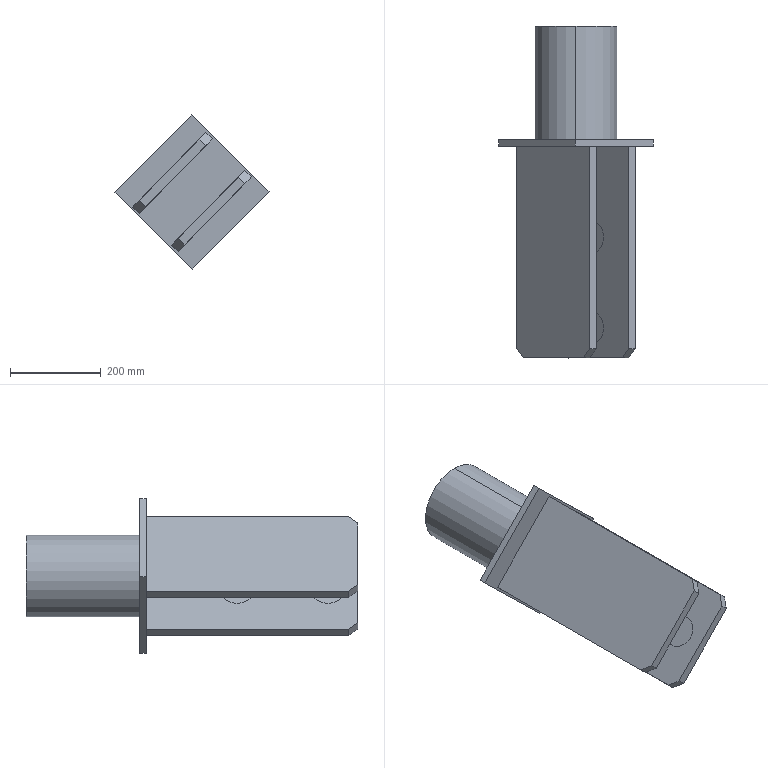Part | SolidWorks | features BaseBody 1 | 1 solid | 35 faces | box 339.392 x 731.247 x 339.392 mm | volume 11422226 mm3 | plane 25 | cylinder 10 | commonest cylinder face diameters 70 x8 180 x2
STEP:
#1=CARTESIAN_POINT('',(14.827,1234.2,-1080.412));
#2=VERTEX_POINT('',#1);
#3=CARTESIAN_POINT('',(63.788,1234.2,-1030.384));
#4=VERTEX_POINT('',#3);
#5=CARTESIAN_POINT('',(39.308,1234.2,-1055.398));
#6=DIRECTION('',(-0.7147,0.,0.6994));
#7=DIRECTION('',(0.6994,0.,0.7147));
#8=AXIS2_PLACEMENT_3D('',#5,#6,#7);
#9=CIRCLE('',#8,35.);
#10=EDGE_CURVE('',#2,#4,#9,.T.);
#11=ORIENTED_EDGE('',*,*,#10,.F.);
#12=CARTESIAN_POINT('',(11.254,1234.2,-1076.915));
#13=VERTEX_POINT('',#12);
#14=CARTESIAN_POINT('',(14.827,1234.2,-1080.412));
#15=DIRECTION('',(-0.7147,0.,0.6994));
#16=VECTOR('',#15,1000.);
#17=LINE('',#14,#16);
#18=EDGE_CURVE('',#2,#13,#17,.T.);
#19=ORIENTED_EDGE('',*,*,#18,.T.);
#20=CARTESIAN_POINT('',(60.215,1234.2,-1026.887));
#21=VERTEX_POINT('',#20);
#22=CARTESIAN_POINT('',(35.734,1234.2,-1051.901));
#23=DIRECTION('',(-0.7147,0.,0.6994));
#24=DIRECTION('',(0.6994,0.,0.7147));
#25=AXIS2_PLACEMENT_3D('',#22,#23,#24);
#26=CIRCLE('',#25,35.);
#27=EDGE_CURVE('',#13,#21,#26,.T.);
#28=ORIENTED_EDGE('',*,*,#27,.T.);
#29=CARTESIAN_POINT('',(63.788,1234.2,-1030.384));
#30=DIRECTION('',(-0.7147,0.,0.6994));
#31=VECTOR('',#30,1000.);
#32=LINE('',#29,#31);
#33=EDGE_CURVE('',#4,#21,#32,.T.);
#34=ORIENTED_EDGE('',*,*,#33,.F.);
#35=EDGE_LOOP('',(#11,#19,#28,#34));
#36=FACE_OUTER_BOUND('',#35,.T.);
#37=CARTESIAN_POINT('',(39.308,1234.2,-1055.398));
#38=DIRECTION('',(-0.7147,0.,0.6994));
#39=DIRECTION('',(0.6994,0.,0.7147));
#40=AXIS2_PLACEMENT_3D('',#37,#38,#39);
#41=CYLINDRICAL_SURFACE('',#40,35.);
#42=ADVANCED_FACE('',(#36),#41,.F.);
#43=CARTESIAN_POINT('',(14.827,1034.2,-1080.412));
#44=VERTEX_POINT('',#43);
#45=CARTESIAN_POINT('',(63.788,1034.2,-1030.384));
#46=VERTEX_POINT('',#45);
#47=CARTESIAN_POINT('',(39.308,1034.2,-1055.398));
#48=DIRECTION('',(-0.7147,0.,0.6994));
#49=DIRECTION('',(0.6994,0.,0.7147));
#50=AXIS2_PLACEMENT_3D('',#47,#48,#49);
#51=CIRCLE('',#50,35.);
#52=EDGE_CURVE('',#44,#46,#51,.T.);
#53=ORIENTED_EDGE('',*,*,#52,.F.);
#54=CARTESIAN_POINT('',(11.254,1034.2,-1076.915));
#55=VERTEX_POINT('',#54);
#56=CARTESIAN_POINT('',(14.827,1034.2,-1080.412));
#57=DIRECTION('',(-0.7147,0.,0.6994));
#58=VECTOR('',#57,1000.);
#59=LINE('',#56,#58);
#60=EDGE_CURVE('',#44,#55,#59,.T.);
#61=ORIENTED_EDGE('',*,*,#60,.T.);
#62=CARTESIAN_POINT('',(60.215,1034.2,-1026.887));
#63=VERTEX_POINT('',#62);
#64=CARTESIAN_POINT('',(35.734,1034.2,-1051.901));
#65=DIRECTION('',(-0.7147,0.,0.6994));
#66=DIRECTION('',(0.6994,0.,0.7147));
#67=AXIS2_PLACEMENT_3D('',#64,#65,#66);
#68=CIRCLE('',#67,35.);
#69=EDGE_CURVE('',#55,#63,#68,.T.);
#70=ORIENTED_EDGE('',*,*,#69,.T.);
#71=CARTESIAN_POINT('',(63.788,1034.2,-1030.384));
#72=DIRECTION('',(-0.7147,0.,0.6994));
#73=VECTOR('',#72,1000.);
#74=LINE('',#71,#73);
#75=EDGE_CURVE('',#46,#63,#74,.T.);
#76=ORIENTED_EDGE('',*,*,#75,.F.);
#77=EDGE_LOOP('',(#53,#61,#70,#76));
#78=FACE_OUTER_BOUND('',#77,.T.);
#79=CARTESIAN_POINT('',(39.308,1034.2,-1055.398));
#80=DIRECTION('',(-0.7147,0.,0.6994));
#81=DIRECTION('',(0.6994,0.,0.7147));
#82=AXIS2_PLACEMENT_3D('',#79,#80,#81);
#83=CYLINDRICAL_SURFACE('',#82,35.);
#84=ADVANCED_FACE('',(#78),#83,.F.);
#85=CARTESIAN_POINT('',(-14.827,1034.2,-953.445));
#86=VERTEX_POINT('',#85);
#87=CARTESIAN_POINT('',(-63.788,1034.2,-1003.473));
#88=VERTEX_POINT('',#87);
#89=CARTESIAN_POINT('',(-39.308,1034.2,-978.459));
#90=DIRECTION('',(0.7147,0.,-0.6994));
#91=DIRECTION('',(-0.6994,0.,-0.7147));
#92=AXIS2_PLACEMENT_3D('',#89,#90,#91);
#93=CIRCLE('',#92,35.);
#94=EDGE_CURVE('',#86,#88,#93,.T.);
#95=ORIENTED_EDGE('',*,*,#94,.F.);
#96=CARTESIAN_POINT('',(-11.254,1034.2,-956.942));
#97=VERTEX_POINT('',#96);
#98=CARTESIAN_POINT('',(-14.827,1034.2,-953.445));
#99=DIRECTION('',(0.7147,0.,-0.6994));
#100=VECTOR('',#99,1000.);
#101=LINE('',#98,#100);
#102=EDGE_CURVE('',#86,#97,#101,.T.);
#103=ORIENTED_EDGE('',*,*,#102,.T.);
#104=CARTESIAN_POINT('',(-60.215,1034.2,-1006.971));
#105=VERTEX_POINT('',#104);
#106=CARTESIAN_POINT('',(-35.734,1034.2,-981.957));
#107=DIRECTION('',(0.7147,0.,-0.6994));
#108=DIRECTION('',(-0.6994,0.,-0.7147));
#109=AXIS2_PLACEMENT_3D('',#106,#107,#108);
#110=CIRCLE('',#109,35.);
#111=EDGE_CURVE('',#97,#105,#110,.T.);
#112=ORIENTED_EDGE('',*,*,#111,.T.);
#113=CARTESIAN_POINT('',(-63.788,1034.2,-1003.473));
#114=DIRECTION('',(0.7147,0.,-0.6994));
#115=VECTOR('',#114,1000.);
#116=LINE('',#113,#115);
#117=EDGE_CURVE('',#88,#105,#116,.T.);
#118=ORIENTED_EDGE('',*,*,#117,.F.);
#119=EDGE_LOOP('',(#95,#103,#112,#118));
#120=FACE_OUTER_BOUND('',#119,.T.);
#121=CARTESIAN_POINT('',(-39.308,1034.2,-978.459));
#122=DIRECTION('',(0.7147,0.,-0.6994));
#123=DIRECTION('',(-0.6994,0.,-0.7147));
#124=AXIS2_PLACEMENT_3D('',#121,#122,#123);
#125=CYLINDRICAL_SURFACE('',#124,35.);
#126=ADVANCED_FACE('',(#120),#125,.F.);
#127=CARTESIAN_POINT('',(-14.827,1234.2,-953.445));
#128=VERTEX_POINT('',#127);
#129=CARTESIAN_POINT('',(-63.788,1234.2,-1003.473));
#130=VERTEX_POINT('',#129);
#131=CARTESIAN_POINT('',(-39.308,1234.2,-978.459));
#132=DIRECTION('',(0.7147,0.,-0.6994));
#133=DIRECTION('',(-0.6994,0.,-0.7147));
#134=AXIS2_PLACEMENT_3D('',#131,#132,#133);
#135=CIRCLE('',#134,35.);
#136=EDGE_CURVE('',#128,#130,#135,.T.);
#137=ORIENTED_EDGE('',*,*,#136,.F.);
#138=CARTESIAN_POINT('',(-11.254,1234.2,-956.942));
#139=VERTEX_POINT('',#138);
#140=CARTESIAN_POINT('',(-14.827,1234.2,-953.445));
#141=DIRECTION('',(0.7147,0.,-0.6994));
#142=VECTOR('',#141,1000.);
#143=LINE('',#140,#142);
#144=EDGE_CURVE('',#128,#139,#143,.T.);
#145=ORIENTED_EDGE('',*,*,#144,.T.);
#146=CARTESIAN_POINT('',(-60.215,1234.2,-1006.971));
#147=VERTEX_POINT('',#146);
#148=CARTESIAN_POINT('',(-35.734,1234.2,-981.957));
#149=DIRECTION('',(0.7147,0.,-0.6994));
#150=DIRECTION('',(-0.6994,0.,-0.7147));
#151=AXIS2_PLACEMENT_3D('',#148,#149,#150);
#152=CIRCLE('',#151,35.);
#153=EDGE_CURVE('',#139,#147,#152,.T.);
#154=ORIENTED_EDGE('',*,*,#153,.T.);
#155=CARTESIAN_POINT('',(-63.788,1234.2,-1003.473));
#156=DIRECTION('',(0.7147,0.,-0.6994));
#157=VECTOR('',#156,1000.);
#158=LINE('',#155,#157);
#159=EDGE_CURVE('',#130,#147,#158,.T.);
#160=ORIENTED_EDGE('',*,*,#159,.F.);
#161=EDGE_LOOP('',(#137,#145,#154,#160));
#162=FACE_OUTER_BOUND('',#161,.T.);
#163=CARTESIAN_POINT('',(-39.308,1234.2,-978.459));
#164=DIRECTION('',(0.7147,0.,-0.6994));
#165=DIRECTION('',(-0.6994,0.,-0.7147));
#166=AXIS2_PLACEMENT_3D('',#163,#164,#165);
#167=CYLINDRICAL_SURFACE('',#166,35.);
#168=ADVANCED_FACE('',(#162),#167,.F.);
#169=CARTESIAN_POINT('',(0.,1699.2,-1106.929));
#170=VERTEX_POINT('',#169);
#171=CARTESIAN_POINT('',(0.,1699.2,-926.929));
#172=VERTEX_POINT('',#171);
#173=CARTESIAN_POINT('',(0.,1699.2,-1016.929));
#174=DIRECTION('',(0.,-1.,0.));
#175=DIRECTION('',(0.,0.,-1.));
#176=AXIS2_PLACEMENT_3D('',#173,#174,#175);
#177=CIRCLE('',#176,90.);
#178=EDGE_CURVE('',#170,#172,#177,.T.);
#179=ORIENTED_EDGE('',*,*,#178,.T.);
#180=CARTESIAN_POINT('',(0.,1449.2,-926.929));
#181=VERTEX_POINT('',#180);
#182=CARTESIAN_POINT('',(0.,1699.2,-926.929));
#183=DIRECTION('',(0.,-1.,0.));
#184=VECTOR('',#183,1000.);
#185=LINE('',#182,#184);
#186=EDGE_CURVE('',#172,#181,#185,.T.);
#187=ORIENTED_EDGE('',*,*,#186,.T.);
#188=CARTESIAN_POINT('',(0.,1449.2,-1106.929));
#189=VERTEX_POINT('',#188);
#190=CARTESIAN_POINT('',(0.,1449.2,-1016.929));
#191=DIRECTION('',(0.,1.,0.));
#192=DIRECTION('',(0.,0.,-1.));
#193=AXIS2_PLACEMENT_3D('',#190,#191,#192);
#194=CIRCLE('',#193,90.);
#195=EDGE_CURVE('',#181,#189,#194,.T.);
#196=ORIENTED_EDGE('',*,*,#195,.T.);
#197=CARTESIAN_POINT('',(0.,1699.2,-1106.929));
#198=DIRECTION('',(0.,-1.,0.));
#199=VECTOR('',#198,1000.);
#200=LINE('',#197,#199);
#201=EDGE_CURVE('',#170,#189,#200,.T.);
#202=ORIENTED_EDGE('',*,*,#201,.F.);
#203=EDGE_LOOP('',(#179,#187,#196,#202));
#204=FACE_OUTER_BOUND('',#203,.T.);
#205=CARTESIAN_POINT('',(0.,1699.2,-1016.929));
#206=DIRECTION('',(0.,-1.,0.));
#207=DIRECTION('',(0.,0.,-1.));
#208=AXIS2_PLACEMENT_3D('',#205,#206,#207);
#209=CYLINDRICAL_SURFACE('',#208,90.);
#210=ADVANCED_FACE('',(#204),#209,.T.);
#211=CARTESIAN_POINT('',(-30.408,987.953,-1148.079));
#212=VERTEX_POINT('',#211);
#213=CARTESIAN_POINT('',(-16.419,967.953,-1133.785));
#214=VERTEX_POINT('',#213);
#215=CARTESIAN_POINT('',(-30.408,987.953,-1148.079));
#216=DIRECTION('',(0.4946,-0.7071,0.5054));
#217=VECTOR('',#216,1000.);
#218=LINE('',#215,#217);
#219=EDGE_CURVE('',#212,#214,#218,.T.);
#220=ORIENTED_EDGE('',*,*,#219,.F.);
#221=CARTESIAN_POINT('',(-30.408,1434.2,-1148.079));
#222=VERTEX_POINT('',#221);
#223=CARTESIAN_POINT('',(-30.408,864.2,-1148.079));
#224=DIRECTION('',(0.,-1.,0.));
#225=VECTOR('',#224,1000.);
#226=LINE('',#223,#225);
#227=EDGE_CURVE('',#222,#212,#226,.T.);
#228=ORIENTED_EDGE('',*,*,#227,.F.);
#229=CARTESIAN_POINT('',(130.464,1434.2,-983.701));
#230=VERTEX_POINT('',#229);
#231=CARTESIAN_POINT('',(-30.408,1434.2,-1148.079));
#232=DIRECTION('',(-0.6994,0.,-0.7147));
#233=VECTOR('',#232,1000.);
#234=LINE('',#231,#233);
#235=EDGE_CURVE('',#230,#222,#234,.T.);
#236=ORIENTED_EDGE('',*,*,#235,.F.);
#237=CARTESIAN_POINT('',(130.464,987.953,-983.701));
#238=VERTEX_POINT('',#237);
#239=CARTESIAN_POINT('',(130.464,864.2,-983.701));
#240=DIRECTION('',(0.,1.,0.));
#241=VECTOR('',#240,1000.);
#242=LINE('',#239,#241);
#243=EDGE_CURVE('',#238,#230,#242,.T.);
#244=ORIENTED_EDGE('',*,*,#243,.F.);
#245=CARTESIAN_POINT('',(116.475,967.953,-997.995));
#246=VERTEX_POINT('',#245);
#247=CARTESIAN_POINT('',(116.475,967.953,-997.995));
#248=DIRECTION('',(0.4946,0.7071,0.5054));
#249=VECTOR('',#248,1000.);
#250=LINE('',#247,#249);
#251=EDGE_CURVE('',#246,#238,#250,.T.);
#252=ORIENTED_EDGE('',*,*,#251,.F.);
#253=CARTESIAN_POINT('',(-30.408,967.953,-1148.079));
#254=DIRECTION('',(0.6994,0.,0.7147));
#255=VECTOR('',#254,1000.);
#256=LINE('',#253,#255);
#257=EDGE_CURVE('',#214,#246,#256,.T.);
#258=ORIENTED_EDGE('',*,*,#257,.F.);
#259=EDGE_LOOP('',(#220,#228,#236,#244,#252,#258));
#260=FACE_OUTER_BOUND('',#259,.T.);
#261=CARTESIAN_POINT('',(-30.408,864.2,-1148.079));
#262=DIRECTION('',(-0.7147,0.,0.6994));
#263=DIRECTION('',(0.6994,0.,0.7147));
#264=AXIS2_PLACEMENT_3D('',#261,#262,#263);
#265=PLANE('',#264);
#266=ADVANCED_FACE('',(#260),#265,.F.);
#267=CARTESIAN_POINT('',(-30.713,967.953,-1119.796));
#268=VERTEX_POINT('',#267);
#269=CARTESIAN_POINT('',(-16.419,967.953,-1133.785));
#270=DIRECTION('',(-0.7147,0.,0.6994));
#271=VECTOR('',#270,1000.);
#272=LINE('',#269,#271);
#273=EDGE_CURVE('',#214,#268,#272,.T.);
#274=ORIENTED_EDGE('',*,*,#273,.F.);
#275=ORIENTED_EDGE('',*,*,#257,.T.);
#276=CARTESIAN_POINT('',(102.182,967.953,-984.006));
#277=VERTEX_POINT('',#276);
#278=CARTESIAN_POINT('',(102.182,967.953,-984.006));
#279=DIRECTION('',(0.7147,0.,-0.6994));
#280=VECTOR('',#279,1000.);
#281=LINE('',#278,#280);
#282=EDGE_CURVE('',#277,#246,#281,.T.);
#283=ORIENTED_EDGE('',*,*,#282,.F.);
#284=CARTESIAN_POINT('',(-30.713,967.953,-1119.796));
#285=DIRECTION('',(0.6994,0.,0.7147));
#286=VECTOR('',#285,1000.);
#287=LINE('',#284,#286);
#288=EDGE_CURVE('',#268,#277,#287,.T.);
#289=ORIENTED_EDGE('',*,*,#288,.F.);
#290=EDGE_LOOP('',(#274,#275,#283,#289));
#291=FACE_OUTER_BOUND('',#290,.T.);
#292=CARTESIAN_POINT('',(155.411,967.953,-1329.934));
#293=DIRECTION('',(0.,1.,0.));
#294=DIRECTION('',(0.,0.,1.));
#295=AXIS2_PLACEMENT_3D('',#292,#293,#294);
#296=PLANE('',#295);
#297=ADVANCED_FACE('',(#291),#296,.F.);
#298=ORIENTED_EDGE('',*,*,#273,.T.);
#299=CARTESIAN_POINT('',(-44.702,987.953,-1134.09));
#300=VERTEX_POINT('',#299);
#301=CARTESIAN_POINT('',(-44.702,987.953,-1134.09));
#302=DIRECTION('',(0.4946,-0.7071,0.5054));
#303=VECTOR('',#302,1000.);
#304=LINE('',#301,#303);
#305=EDGE_CURVE('',#300,#268,#304,.T.);
#306=ORIENTED_EDGE('',*,*,#305,.F.);
#307=CARTESIAN_POINT('',(-30.408,987.953,-1148.079));
#308=DIRECTION('',(-0.7147,0.,0.6994));
#309=VECTOR('',#308,1000.);
#310=LINE('',#307,#309);
#311=EDGE_CURVE('',#212,#300,#310,.T.);
#312=ORIENTED_EDGE('',*,*,#311,.F.);
#313=ORIENTED_EDGE('',*,*,#219,.T.);
#314=EDGE_LOOP('',(#298,#306,#312,#313));
#315=FACE_OUTER_BOUND('',#314,.T.);
#316=CARTESIAN_POINT('',(-30.408,987.953,-1148.079));
#317=DIRECTION('',(0.4946,0.7071,0.5054));
#318=DIRECTION('',(0.,-0.5815,0.8136));
#319=AXIS2_PLACEMENT_3D('',#316,#317,#318);
#320=PLANE('',#319);
#321=ADVANCED_FACE('',(#315),#320,.F.);
#322=ORIENTED_EDGE('',*,*,#311,.T.);
#323=CARTESIAN_POINT('',(-44.702,1434.2,-1134.09));
#324=VERTEX_POINT('',#323);
#325=CARTESIAN_POINT('',(-44.702,864.2,-1134.09));
#326=DIRECTION('',(0.,-1.,0.));
#327=VECTOR('',#326,1000.);
#328=LINE('',#325,#327);
#329=EDGE_CURVE('',#324,#300,#328,.T.);
#330=ORIENTED_EDGE('',*,*,#329,.F.);
#331=CARTESIAN_POINT('',(-30.408,1434.2,-1148.079));
#332=DIRECTION('',(-0.7147,0.,0.6994));
#333=VECTOR('',#332,1000.);
#334=LINE('',#331,#333);
#335=EDGE_CURVE('',#222,#324,#334,.T.);
#336=ORIENTED_EDGE('',*,*,#335,.F.);
#337=ORIENTED_EDGE('',*,*,#227,.T.);
#338=EDGE_LOOP('',(#322,#330,#336,#337));
#339=FACE_OUTER_BOUND('',#338,.T.);
#340=CARTESIAN_POINT('',(-30.408,864.2,-1148.079));
#341=DIRECTION('',(0.6994,0.,0.7147));
#342=DIRECTION('',(0.7147,0.,-0.6994));
#343=AXIS2_PLACEMENT_3D('',#340,#341,#342);
#344=PLANE('',#343);
#345=ADVANCED_FACE('',(#339),#344,.F.);
#346=CARTESIAN_POINT('',(-130.464,1434.2,-1050.157));
#347=VERTEX_POINT('',#346);
#348=CARTESIAN_POINT('',(30.408,1434.2,-885.779));
#349=VERTEX_POINT('',#348);
#350=CARTESIAN_POINT('',(-130.464,1434.2,-1050.157));
#351=DIRECTION('',(0.6994,0.,0.7147));
#352=VECTOR('',#351,1000.);
#353=LINE('',#350,#352);
#354=EDGE_CURVE('',#347,#349,#353,.T.);
#355=ORIENTED_EDGE('',*,*,#354,.T.);
#356=CARTESIAN_POINT('',(44.702,1434.2,-899.767));
#357=VERTEX_POINT('',#356);
#358=CARTESIAN_POINT('',(30.408,1434.2,-885.779));
#359=DIRECTION('',(0.7147,0.,-0.6994));
#360=VECTOR('',#359,1000.);
#361=LINE('',#358,#360);
#362=EDGE_CURVE('',#349,#357,#361,.T.);
#363=ORIENTED_EDGE('',*,*,#362,.T.);
#364=CARTESIAN_POINT('',(-116.17,1434.2,-1064.146));
#365=VERTEX_POINT('',#364);
#366=CARTESIAN_POINT('',(44.702,1434.2,-899.767));
#367=DIRECTION('',(-0.6994,0.,-0.7147));
#368=VECTOR('',#367,1000.);
#369=LINE('',#366,#368);
#370=EDGE_CURVE('',#357,#365,#369,.T.);
#371=ORIENTED_EDGE('',*,*,#370,.T.);
#372=CARTESIAN_POINT('',(-116.17,1434.2,-1064.146));
#373=DIRECTION('',(-0.7147,0.,0.6994));
#374=VECTOR('',#373,1000.);
#375=LINE('',#372,#374);
#376=EDGE_CURVE('',#365,#347,#375,.T.);
#377=ORIENTED_EDGE('',*,*,#376,.T.);
#378=EDGE_LOOP('',(#355,#363,#371,#377));
#379=FACE_BOUND('',#378,.T.);
#380=CARTESIAN_POINT('',(-1.829,1434.2,-847.233));
#381=VERTEX_POINT('',#380);
#382=CARTESIAN_POINT('',(-169.696,1434.2,-1018.758));
#383=VERTEX_POINT('',#382);
#384=CARTESIAN_POINT('',(-1.829,1434.2,-847.233));
#385=DIRECTION('',(-0.6994,0.,-0.7147));
#386=VECTOR('',#385,1000.);
#387=LINE('',#384,#386);
#388=EDGE_CURVE('',#381,#383,#387,.T.);
#389=ORIENTED_EDGE('',*,*,#388,.T.);
#390=CARTESIAN_POINT('',(1.829,1434.2,-1186.625));
#391=VERTEX_POINT('',#390);
#392=CARTESIAN_POINT('',(-169.696,1434.2,-1018.758));
#393=DIRECTION('',(0.7147,0.,-0.6994));
#394=VECTOR('',#393,1000.);
#395=LINE('',#392,#394);
#396=EDGE_CURVE('',#383,#391,#395,.T.);
#397=ORIENTED_EDGE('',*,*,#396,.T.);
#398=CARTESIAN_POINT('',(169.696,1434.2,-1015.1));
#399=VERTEX_POINT('',#398);
#400=CARTESIAN_POINT('',(1.829,1434.2,-1186.625));
#401=DIRECTION('',(0.6994,0.,0.7147));
#402=VECTOR('',#401,1000.);
#403=LINE('',#400,#402);
#404=EDGE_CURVE('',#391,#399,#403,.T.);
#405=ORIENTED_EDGE('',*,*,#404,.T.);
#406=CARTESIAN_POINT('',(169.696,1434.2,-1015.1));
#407=DIRECTION('',(-0.7147,0.,0.6994));
#408=VECTOR('',#407,1000.);
#409=LINE('',#406,#408);
#410=EDGE_CURVE('',#399,#381,#409,.T.);
#411=ORIENTED_EDGE('',*,*,#410,.T.);
#412=EDGE_LOOP('',(#389,#397,#405,#411));
#413=FACE_OUTER_BOUND('',#412,.T.);
#414=ORIENTED_EDGE('',*,*,#335,.T.);
#415=CARTESIAN_POINT('',(116.17,1434.2,-969.712));
#416=VERTEX_POINT('',#415);
#417=CARTESIAN_POINT('',(-44.702,1434.2,-1134.09));
#418=DIRECTION('',(0.6994,0.,0.7147));
#419=VECTOR('',#418,1000.);
#420=LINE('',#417,#419);
#421=EDGE_CURVE('',#324,#416,#420,.T.);
#422=ORIENTED_EDGE('',*,*,#421,.T.);
#423=CARTESIAN_POINT('',(116.17,1434.2,-969.712));
#424=DIRECTION('',(0.7147,0.,-0.6994));
#425=VECTOR('',#424,1000.);
#426=LINE('',#423,#425);
#427=EDGE_CURVE('',#416,#230,#426,.T.);
#428=ORIENTED_EDGE('',*,*,#427,.T.);
#429=ORIENTED_EDGE('',*,*,#235,.T.);
#430=EDGE_LOOP('',(#414,#422,#428,#429));
#431=FACE_BOUND('',#430,.T.);
#432=CARTESIAN_POINT('',(0.,1434.2,-1016.929));
#433=DIRECTION('',(0.,-1.,0.));
#434=DIRECTION('',(0.,0.,-1.));
#435=AXIS2_PLACEMENT_3D('',#432,#433,#434);
#436=PLANE('',#435);
#437=ADVANCED_FACE('',(#379,#413,#431),#436,.T.);
#438=CARTESIAN_POINT('',(116.17,987.953,-969.712));
#439=VERTEX_POINT('',#438);
#440=CARTESIAN_POINT('',(130.464,987.953,-983.701));
#441=DIRECTION('',(-0.7147,0.,0.6994));
#442=VECTOR('',#441,1000.);
#443=LINE('',#440,#442);
#444=EDGE_CURVE('',#238,#439,#443,.T.);
#445=ORIENTED_EDGE('',*,*,#444,.F.);
#446=ORIENTED_EDGE('',*,*,#243,.T.);
#447=ORIENTED_EDGE('',*,*,#427,.F.);
#448=CARTESIAN_POINT('',(116.17,864.2,-969.712));
#449=DIRECTION('',(0.,1.,0.));
#450=VECTOR('',#449,1000.);
#451=LINE('',#448,#450);
#452=EDGE_CURVE('',#439,#416,#451,.T.);
#453=ORIENTED_EDGE('',*,*,#452,.F.);
#454=EDGE_LOOP('',(#445,#446,#447,#453));
#455=FACE_OUTER_BOUND('',#454,.T.);
#456=CARTESIAN_POINT('',(130.464,864.2,-983.701));
#457=DIRECTION('',(-0.6994,0.,-0.7147));
#458=DIRECTION('',(-0.7147,0.,0.6994));
#459=AXIS2_PLACEMENT_3D('',#456,#457,#458);
#460=PLANE('',#459);
#461=ADVANCED_FACE('',(#455),#460,.F.);
#462=ORIENTED_EDGE('',*,*,#444,.T.);
#463=CARTESIAN_POINT('',(102.182,967.953,-984.006));
#464=DIRECTION('',(0.4946,0.7071,0.5054));
#465=VECTOR('',#464,1000.);
#466=LINE('',#463,#465);
#467=EDGE_CURVE('',#277,#439,#466,.T.);
#468=ORIENTED_EDGE('',*,*,#467,.F.);
#469=ORIENTED_EDGE('',*,*,#282,.T.);
#470=ORIENTED_EDGE('',*,*,#251,.T.);
#471=EDGE_LOOP('',(#462,#468,#469,#470));
#472=FACE_OUTER_BOUND('',#471,.T.);
#473=CARTESIAN_POINT('',(302.294,967.953,-1179.85));
#474=DIRECTION('',(-0.4946,0.7071,-0.5054));
#475=DIRECTION('',(0.,0.5815,0.8136));
#476=AXIS2_PLACEMENT_3D('',#473,#474,#475);
#477=PLANE('',#476);
#478=ADVANCED_FACE('',(#472),#477,.F.);
#479=CARTESIAN_POINT('',(35.734,1234.2,-1051.901));
#480=DIRECTION('',(-0.7147,0.,0.6994));
#481=DIRECTION('',(0.6994,0.,0.7147));
#482=AXIS2_PLACEMENT_3D('',#479,#480,#481);
#483=CIRCLE('',#482,35.);
#484=EDGE_CURVE('',#21,#13,#483,.T.);
#485=ORIENTED_EDGE('',*,*,#484,.F.);
#486=ORIENTED_EDGE('',*,*,#27,.F.);
#487=EDGE_LOOP('',(#485,#486));
#488=FACE_BOUND('',#487,.T.);
#489=ORIENTED_EDGE('',*,*,#305,.T.);
#490=ORIENTED_EDGE('',*,*,#288,.T.);
#491=ORIENTED_EDGE('',*,*,#467,.T.);
#492=ORIENTED_EDGE('',*,*,#452,.T.);
#493=ORIENTED_EDGE('',*,*,#421,.F.);
#494=ORIENTED_EDGE('',*,*,#329,.T.);
#495=EDGE_LOOP('',(#489,#490,#491,#492,#493,#494));
#496=FACE_OUTER_BOUND('',#495,.T.);
#497=CARTESIAN_POINT('',(35.734,1034.2,-1051.901));
#498=DIRECTION('',(-0.7147,0.,0.6994));
#499=DIRECTION('',(0.6994,0.,0.7147));
#500=AXIS2_PLACEMENT_3D('',#497,#498,#499);
#501=CIRCLE('',#500,35.);
#502=EDGE_CURVE('',#63,#55,#501,.T.);
#503=ORIENTED_EDGE('',*,*,#502,.F.);
#504=ORIENTED_EDGE('',*,*,#69,.F.);
#505=EDGE_LOOP('',(#503,#504));
#506=FACE_BOUND('',#505,.T.);
#507=CARTESIAN_POINT('',(-44.702,864.2,-1134.09));
#508=DIRECTION('',(0.7147,0.,-0.6994));
#509=DIRECTION('',(-0.6994,0.,-0.7147));
#510=AXIS2_PLACEMENT_3D('',#507,#508,#509);
#511=PLANE('',#510);
#512=ADVANCED_FACE('',(#488,#496,#506),#511,.F.);
#513=CARTESIAN_POINT('',(44.702,987.953,-899.767));
#514=VERTEX_POINT('',#513);
#515=CARTESIAN_POINT('',(30.408,987.953,-885.779));
#516=VERTEX_POINT('',#515);
#517=CARTESIAN_POINT('',(30.408,987.953,-885.779));
#518=DIRECTION('',(-0.7147,0.,0.6994));
#519=VECTOR('',#518,1000.);
#520=LINE('',#517,#519);
#521=EDGE_CURVE('',#514,#516,#520,.T.);
#522=ORIENTED_EDGE('',*,*,#521,.F.);
#523=CARTESIAN_POINT('',(44.702,864.2,-899.767));
#524=DIRECTION('',(0.,-1.,0.));
#525=VECTOR('',#524,1000.);
#526=LINE('',#523,#525);
#527=EDGE_CURVE('',#357,#514,#526,.T.);
#528=ORIENTED_EDGE('',*,*,#527,.F.);
#529=ORIENTED_EDGE('',*,*,#362,.F.);
#530=CARTESIAN_POINT('',(30.408,864.2,-885.779));
#531=DIRECTION('',(0.,1.,0.));
#532=VECTOR('',#531,1000.);
#533=LINE('',#530,#532);
#534=EDGE_CURVE('',#516,#349,#533,.T.);
#535=ORIENTED_EDGE('',*,*,#534,.F.);
#536=EDGE_LOOP('',(#522,#528,#529,#535));
#537=FACE_OUTER_BOUND('',#536,.T.);
#538=CARTESIAN_POINT('',(30.408,864.2,-885.779));
#539=DIRECTION('',(-0.6994,0.,-0.7147));
#540=DIRECTION('',(-0.7147,0.,0.6994));
#541=AXIS2_PLACEMENT_3D('',#538,#539,#540);
#542=PLANE('',#541);
#543=ADVANCED_FACE('',(#537),#542,.F.);
#544=CARTESIAN_POINT('',(16.419,967.953,-900.072));
#545=VERTEX_POINT('',#544);
#546=CARTESIAN_POINT('',(30.408,987.953,-885.779));
#547=DIRECTION('',(-0.4946,-0.7071,-0.5054));
#548=VECTOR('',#547,1000.);
#549=LINE('',#546,#548);
#550=EDGE_CURVE('',#516,#545,#549,.T.);
#551=ORIENTED_EDGE('',*,*,#550,.F.);
#552=ORIENTED_EDGE('',*,*,#534,.T.);
#553=ORIENTED_EDGE('',*,*,#354,.F.);
#554=CARTESIAN_POINT('',(-130.464,987.953,-1050.157));
#555=VERTEX_POINT('',#554);
#556=CARTESIAN_POINT('',(-130.464,864.2,-1050.157));
#557=DIRECTION('',(0.,1.,0.));
#558=VECTOR('',#557,1000.);
#559=LINE('',#556,#558);
#560=EDGE_CURVE('',#555,#347,#559,.T.);
#561=ORIENTED_EDGE('',*,*,#560,.F.);
#562=CARTESIAN_POINT('',(-116.475,967.953,-1035.863));
#563=VERTEX_POINT('',#562);
#564=CARTESIAN_POINT('',(-116.475,967.953,-1035.863));
#565=DIRECTION('',(-0.4946,0.7071,-0.5054));
#566=VECTOR('',#565,1000.);
#567=LINE('',#564,#566);
#568=EDGE_CURVE('',#563,#555,#567,.T.);
#569=ORIENTED_EDGE('',*,*,#568,.F.);
#570=CARTESIAN_POINT('',(-130.464,967.953,-1050.157));
#571=DIRECTION('',(-0.6994,0.,-0.7147));
#572=VECTOR('',#571,1000.);
#573=LINE('',#570,#572);
#574=EDGE_CURVE('',#545,#563,#573,.T.);
#575=ORIENTED_EDGE('',*,*,#574,.F.);
#576=EDGE_LOOP('',(#551,#552,#553,#561,#569,#575));
#577=FACE_OUTER_BOUND('',#576,.T.);
#578=CARTESIAN_POINT('',(-130.464,864.2,-1050.157));
#579=DIRECTION('',(0.7147,0.,-0.6994));
#580=DIRECTION('',(-0.6994,0.,-0.7147));
#581=AXIS2_PLACEMENT_3D('',#578,#579,#580);
#582=PLANE('',#581);
#583=ADVANCED_FACE('',(#577),#582,.F.);
#584=CARTESIAN_POINT('',(-116.17,987.953,-1064.146));
#585=VERTEX_POINT('',#584);
#586=CARTESIAN_POINT('',(-130.464,987.953,-1050.157));
#587=DIRECTION('',(0.7147,0.,-0.6994));
#588=VECTOR('',#587,1000.);
#589=LINE('',#586,#588);
#590=EDGE_CURVE('',#555,#585,#589,.T.);
#591=ORIENTED_EDGE('',*,*,#590,.F.);
#592=ORIENTED_EDGE('',*,*,#560,.T.);
#593=ORIENTED_EDGE('',*,*,#376,.F.);
#594=CARTESIAN_POINT('',(-116.17,864.2,-1064.146));
#595=DIRECTION('',(0.,1.,0.));
#596=VECTOR('',#595,1000.);
#597=LINE('',#594,#596);
#598=EDGE_CURVE('',#585,#365,#597,.T.);
#599=ORIENTED_EDGE('',*,*,#598,.F.);
#600=EDGE_LOOP('',(#591,#592,#593,#599));
#601=FACE_OUTER_BOUND('',#600,.T.);
#602=CARTESIAN_POINT('',(-130.464,864.2,-1050.157));
#603=DIRECTION('',(0.6994,0.,0.7147));
#604=DIRECTION('',(0.7147,0.,-0.6994));
#605=AXIS2_PLACEMENT_3D('',#602,#603,#604);
#606=PLANE('',#605);
#607=ADVANCED_FACE('',(#601),#606,.F.);
#608=CARTESIAN_POINT('',(30.713,967.953,-914.061));
#609=VERTEX_POINT('',#608);
#610=CARTESIAN_POINT('',(30.713,967.953,-914.061));
#611=DIRECTION('',(0.4946,0.7071,0.5054));
#612=VECTOR('',#611,1000.);
#613=LINE('',#610,#612);
#614=EDGE_CURVE('',#609,#514,#613,.T.);
#615=ORIENTED_EDGE('',*,*,#614,.F.);
#616=CARTESIAN_POINT('',(-102.182,967.953,-1049.852));
#617=VERTEX_POINT('',#616);
#618=CARTESIAN_POINT('',(-116.17,967.953,-1064.146));
#619=DIRECTION('',(0.6994,0.,0.7147));
#620=VECTOR('',#619,1000.);
#621=LINE('',#618,#620);
#622=EDGE_CURVE('',#617,#609,#621,.T.);
#623=ORIENTED_EDGE('',*,*,#622,.F.);
#624=CARTESIAN_POINT('',(-116.17,987.953,-1064.146));
#625=DIRECTION('',(0.4946,-0.7071,0.5054));
#626=VECTOR('',#625,1000.);
#627=LINE('',#624,#626);
#628=EDGE_CURVE('',#585,#617,#627,.T.);
#629=ORIENTED_EDGE('',*,*,#628,.F.);
#630=ORIENTED_EDGE('',*,*,#598,.T.);
#631=ORIENTED_EDGE('',*,*,#370,.F.);
#632=ORIENTED_EDGE('',*,*,#527,.T.);
#633=EDGE_LOOP('',(#615,#623,#629,#630,#631,#632));
#634=FACE_OUTER_BOUND('',#633,.T.);
#635=CARTESIAN_POINT('',(-35.734,1034.2,-981.957));
#636=DIRECTION('',(0.7147,0.,-0.6994));
#637=DIRECTION('',(-0.6994,0.,-0.7147));
#638=AXIS2_PLACEMENT_3D('',#635,#636,#637);
#639=CIRCLE('',#638,35.);
#640=EDGE_CURVE('',#105,#97,#639,.T.);
#641=ORIENTED_EDGE('',*,*,#640,.F.);
#642=ORIENTED_EDGE('',*,*,#111,.F.);
#643=EDGE_LOOP('',(#641,#642));
#644=FACE_BOUND('',#643,.T.);
#645=CARTESIAN_POINT('',(-35.734,1234.2,-981.957));
#646=DIRECTION('',(0.7147,0.,-0.6994));
#647=DIRECTION('',(-0.6994,0.,-0.7147));
#648=AXIS2_PLACEMENT_3D('',#645,#646,#647);
#649=CIRCLE('',#648,35.);
#650=EDGE_CURVE('',#147,#139,#649,.T.);
#651=ORIENTED_EDGE('',*,*,#650,.F.);
#652=ORIENTED_EDGE('',*,*,#153,.F.);
#653=EDGE_LOOP('',(#651,#652));
#654=FACE_BOUND('',#653,.T.);
#655=CARTESIAN_POINT('',(-116.17,864.2,-1064.146));
#656=DIRECTION('',(-0.7147,0.,0.6994));
#657=DIRECTION('',(0.6994,0.,0.7147));
#658=AXIS2_PLACEMENT_3D('',#655,#656,#657);
#659=PLANE('',#658);
#660=ADVANCED_FACE('',(#634,#644,#654),#659,.F.);
#661=CARTESIAN_POINT('',(1.829,1449.2,-1186.625));
#662=VERTEX_POINT('',#661);
#663=CARTESIAN_POINT('',(1.829,1434.2,-1186.625));
#664=DIRECTION('',(0.,1.,0.));
#665=VECTOR('',#664,1000.);
#666=LINE('',#663,#665);
#667=EDGE_CURVE('',#391,#662,#666,.T.);
#668=ORIENTED_EDGE('',*,*,#667,.F.);
#669=ORIENTED_EDGE('',*,*,#396,.F.);
#670=CARTESIAN_POINT('',(-169.696,1449.2,-1018.758));
#671=VERTEX_POINT('',#670);
#672=CARTESIAN_POINT('',(-169.696,1434.2,-1018.758));
#673=DIRECTION('',(0.,-1.,0.));
#674=VECTOR('',#673,1000.);
#675=LINE('',#672,#674);
#676=EDGE_CURVE('',#671,#383,#675,.T.);
#677=ORIENTED_EDGE('',*,*,#676,.F.);
#678=CARTESIAN_POINT('',(1.829,1449.2,-1186.625));
#679=DIRECTION('',(-0.7147,0.,0.6994));
#680=VECTOR('',#679,1000.);
#681=LINE('',#678,#680);
#682=EDGE_CURVE('',#662,#671,#681,.T.);
#683=ORIENTED_EDGE('',*,*,#682,.F.);
#684=EDGE_LOOP('',(#668,#669,#677,#683));
#685=FACE_OUTER_BOUND('',#684,.T.);
#686=CARTESIAN_POINT('',(1.829,1434.2,-1186.625));
#687=DIRECTION('',(0.6994,0.,0.7147));
#688=DIRECTION('',(0.7147,0.,-0.6994));
#689=AXIS2_PLACEMENT_3D('',#686,#687,#688);
#690=PLANE('',#689);
#691=ADVANCED_FACE('',(#685),#690,.F.);
#692=ORIENTED_EDGE('',*,*,#676,.T.);
#693=ORIENTED_EDGE('',*,*,#388,.F.);
#694=CARTESIAN_POINT('',(-1.829,1449.2,-847.233));
#695=VERTEX_POINT('',#694);
#696=CARTESIAN_POINT('',(-1.829,1434.2,-847.233));
#697=DIRECTION('',(0.,-1.,0.));
#698=VECTOR('',#697,1000.);
#699=LINE('',#696,#698);
#700=EDGE_CURVE('',#695,#381,#699,.T.);
#701=ORIENTED_EDGE('',*,*,#700,.F.);
#702=CARTESIAN_POINT('',(-169.696,1449.2,-1018.758));
#703=DIRECTION('',(0.6994,0.,0.7147));
#704=VECTOR('',#703,1000.);
#705=LINE('',#702,#704);
#706=EDGE_CURVE('',#671,#695,#705,.T.);
#707=ORIENTED_EDGE('',*,*,#706,.F.);
#708=EDGE_LOOP('',(#692,#693,#701,#707));
#709=FACE_OUTER_BOUND('',#708,.T.);
#710=CARTESIAN_POINT('',(-169.696,1434.2,-1018.758));
#711=DIRECTION('',(0.7147,0.,-0.6994));
#712=DIRECTION('',(-0.6994,0.,-0.7147));
#713=AXIS2_PLACEMENT_3D('',#710,#711,#712);
#714=PLANE('',#713);
#715=ADVANCED_FACE('',(#709),#714,.F.);
#716=ORIENTED_EDGE('',*,*,#700,.T.);
#717=ORIENTED_EDGE('',*,*,#410,.F.);
#718=CARTESIAN_POINT('',(169.696,1449.2,-1015.1));
#719=VERTEX_POINT('',#718);
#720=CARTESIAN_POINT('',(169.696,1434.2,-1015.1));
#721=DIRECTION('',(0.,-1.,0.));
#722=VECTOR('',#721,1000.);
#723=LINE('',#720,#722);
#724=EDGE_CURVE('',#719,#399,#723,.T.);
#725=ORIENTED_EDGE('',*,*,#724,.F.);
#726=CARTESIAN_POINT('',(169.696,1449.2,-1015.1));
#727=DIRECTION('',(0.7147,0.,-0.6994));
#728=VECTOR('',#727,1000.);
#729=LINE('',#726,#728);
#730=EDGE_CURVE('',#695,#719,#729,.T.);
#731=ORIENTED_EDGE('',*,*,#730,.F.);
#732=EDGE_LOOP('',(#716,#717,#725,#731));
#733=FACE_OUTER_BOUND('',#732,.T.);
#734=CARTESIAN_POINT('',(169.696,1434.2,-1015.1));
#735=DIRECTION('',(-0.6994,0.,-0.7147));
#736=DIRECTION('',(-0.7147,0.,0.6994));
#737=AXIS2_PLACEMENT_3D('',#734,#735,#736);
#738=PLANE('',#737);
#739=ADVANCED_FACE('',(#733),#738,.F.);
#740=ORIENTED_EDGE('',*,*,#724,.T.);
#741=ORIENTED_EDGE('',*,*,#404,.F.);
#742=ORIENTED_EDGE('',*,*,#667,.T.);
#743=CARTESIAN_POINT('',(1.829,1449.2,-1186.625));
#744=DIRECTION('',(-0.6994,0.,-0.7147));
#745=VECTOR('',#744,1000.);
#746=LINE('',#743,#745);
#747=EDGE_CURVE('',#719,#662,#746,.T.);
#748=ORIENTED_EDGE('',*,*,#747,.F.);
#749=EDGE_LOOP('',(#740,#741,#742,#748));
#750=FACE_OUTER_BOUND('',#749,.T.);
#751=CARTESIAN_POINT('',(1.829,1434.2,-1186.625));
#752=DIRECTION('',(-0.7147,0.,0.6994));
#753=DIRECTION('',(0.6994,0.,0.7147));
#754=AXIS2_PLACEMENT_3D('',#751,#752,#753);
#755=PLANE('',#754);
#756=ADVANCED_FACE('',(#750),#755,.F.);
#757=ORIENTED_EDGE('',*,*,#18,.F.);
#758=CARTESIAN_POINT('',(39.308,1234.2,-1055.398));
#759=DIRECTION('',(-0.7147,0.,0.6994));
#760=DIRECTION('',(0.6994,0.,0.7147));
#761=AXIS2_PLACEMENT_3D('',#758,#759,#760);
#762=CIRCLE('',#761,35.);
#763=EDGE_CURVE('',#4,#2,#762,.T.);
#764=ORIENTED_EDGE('',*,*,#763,.F.);
#765=ORIENTED_EDGE('',*,*,#33,.T.);
#766=ORIENTED_EDGE('',*,*,#484,.T.);
#767=EDGE_LOOP('',(#757,#764,#765,#766));
#768=FACE_OUTER_BOUND('',#767,.T.);
#769=CARTESIAN_POINT('',(39.308,1234.2,-1055.398));
#770=DIRECTION('',(-0.7147,0.,0.6994));
#771=DIRECTION('',(0.6994,0.,0.7147));
#772=AXIS2_PLACEMENT_3D('',#769,#770,#771);
#773=CYLINDRICAL_SURFACE('',#772,35.);
#774=ADVANCED_FACE('',(#768),#773,.F.);
#775=ORIENTED_EDGE('',*,*,#60,.F.);
#776=CARTESIAN_POINT('',(39.308,1034.2,-1055.398));
#777=DIRECTION('',(-0.7147,0.,0.6994));
#778=DIRECTION('',(0.6994,0.,0.7147));
#779=AXIS2_PLACEMENT_3D('',#776,#777,#778);
#780=CIRCLE('',#779,35.);
#781=EDGE_CURVE('',#46,#44,#780,.T.);
#782=ORIENTED_EDGE('',*,*,#781,.F.);
#783=ORIENTED_EDGE('',*,*,#75,.T.);
#784=ORIENTED_EDGE('',*,*,#502,.T.);
#785=EDGE_LOOP('',(#775,#782,#783,#784));
#786=FACE_OUTER_BOUND('',#785,.T.);
#787=CARTESIAN_POINT('',(39.308,1034.2,-1055.398));
#788=DIRECTION('',(-0.7147,0.,0.6994));
#789=DIRECTION('',(0.6994,0.,0.7147));
#790=AXIS2_PLACEMENT_3D('',#787,#788,#789);
#791=CYLINDRICAL_SURFACE('',#790,35.);
#792=ADVANCED_FACE('',(#786),#791,.F.);
#793=ORIENTED_EDGE('',*,*,#521,.T.);
#794=ORIENTED_EDGE('',*,*,#550,.T.);
#795=CARTESIAN_POINT('',(30.713,967.953,-914.061));
#796=DIRECTION('',(-0.7147,0.,0.6994));
#797=VECTOR('',#796,1000.);
#798=LINE('',#795,#797);
#799=EDGE_CURVE('',#609,#545,#798,.T.);
#800=ORIENTED_EDGE('',*,*,#799,.F.);
#801=ORIENTED_EDGE('',*,*,#614,.T.);
#802=EDGE_LOOP('',(#793,#794,#800,#801));
#803=FACE_OUTER_BOUND('',#802,.T.);
#804=CARTESIAN_POINT('',(302.294,967.953,-1179.85));
#805=DIRECTION('',(-0.4946,0.7071,-0.5054));
#806=DIRECTION('',(0.,0.5815,0.8136));
#807=AXIS2_PLACEMENT_3D('',#804,#805,#806);
#808=PLANE('',#807);
#809=ADVANCED_FACE('',(#803),#808,.F.);
#810=ORIENTED_EDGE('',*,*,#799,.T.);
#811=ORIENTED_EDGE('',*,*,#574,.T.);
#812=CARTESIAN_POINT('',(-102.182,967.953,-1049.852));
#813=DIRECTION('',(-0.7147,0.,0.6994));
#814=VECTOR('',#813,1000.);
#815=LINE('',#812,#814);
#816=EDGE_CURVE('',#617,#563,#815,.T.);
#817=ORIENTED_EDGE('',*,*,#816,.F.);
#818=ORIENTED_EDGE('',*,*,#622,.T.);
#819=EDGE_LOOP('',(#810,#811,#817,#818));
#820=FACE_OUTER_BOUND('',#819,.T.);
#821=CARTESIAN_POINT('',(155.411,967.953,-1329.934));
#822=DIRECTION('',(0.,1.,0.));
#823=DIRECTION('',(0.,0.,1.));
#824=AXIS2_PLACEMENT_3D('',#821,#822,#823);
#825=PLANE('',#824);
#826=ADVANCED_FACE('',(#820),#825,.F.);
#827=ORIENTED_EDGE('',*,*,#816,.T.);
#828=ORIENTED_EDGE('',*,*,#568,.T.);
#829=ORIENTED_EDGE('',*,*,#590,.T.);
#830=ORIENTED_EDGE('',*,*,#628,.T.);
#831=EDGE_LOOP('',(#827,#828,#829,#830));
#832=FACE_OUTER_BOUND('',#831,.T.);
#833=CARTESIAN_POINT('',(-130.464,987.953,-1050.157));
#834=DIRECTION('',(0.4946,0.7071,0.5054));
#835=DIRECTION('',(0.,-0.5815,0.8136));
#836=AXIS2_PLACEMENT_3D('',#833,#834,#835);
#837=PLANE('',#836);
#838=ADVANCED_FACE('',(#832),#837,.F.);
#839=ORIENTED_EDGE('',*,*,#102,.F.);
#840=CARTESIAN_POINT('',(-39.308,1034.2,-978.459));
#841=DIRECTION('',(0.7147,0.,-0.6994));
#842=DIRECTION('',(-0.6994,0.,-0.7147));
#843=AXIS2_PLACEMENT_3D('',#840,#841,#842);
#844=CIRCLE('',#843,35.);
#845=EDGE_CURVE('',#88,#86,#844,.T.);
#846=ORIENTED_EDGE('',*,*,#845,.F.);
#847=ORIENTED_EDGE('',*,*,#117,.T.);
#848=ORIENTED_EDGE('',*,*,#640,.T.);
#849=EDGE_LOOP('',(#839,#846,#847,#848));
#850=FACE_OUTER_BOUND('',#849,.T.);
#851=CARTESIAN_POINT('',(-39.308,1034.2,-978.459));
#852=DIRECTION('',(0.7147,0.,-0.6994));
#853=DIRECTION('',(-0.6994,0.,-0.7147));
#854=AXIS2_PLACEMENT_3D('',#851,#852,#853);
#855=CYLINDRICAL_SURFACE('',#854,35.);
#856=ADVANCED_FACE('',(#850),#855,.F.);
#857=ORIENTED_EDGE('',*,*,#144,.F.);
#858=CARTESIAN_POINT('',(-39.308,1234.2,-978.459));
#859=DIRECTION('',(0.7147,0.,-0.6994));
#860=DIRECTION('',(-0.6994,0.,-0.7147));
#861=AXIS2_PLACEMENT_3D('',#858,#859,#860);
#862=CIRCLE('',#861,35.);
#863=EDGE_CURVE('',#130,#128,#862,.T.);
#864=ORIENTED_EDGE('',*,*,#863,.F.);
#865=ORIENTED_EDGE('',*,*,#159,.T.);
#866=ORIENTED_EDGE('',*,*,#650,.T.);
#867=EDGE_LOOP('',(#857,#864,#865,#866));
#868=FACE_OUTER_BOUND('',#867,.T.);
#869=CARTESIAN_POINT('',(-39.308,1234.2,-978.459));
#870=DIRECTION('',(0.7147,0.,-0.6994));
#871=DIRECTION('',(-0.6994,0.,-0.7147));
#872=AXIS2_PLACEMENT_3D('',#869,#870,#871);
#873=CYLINDRICAL_SURFACE('',#872,35.);
#874=ADVANCED_FACE('',(#868),#873,.F.);
#875=CARTESIAN_POINT('',(0.,1449.2,-1016.929));
#876=DIRECTION('',(0.,1.,0.));
#877=DIRECTION('',(0.,0.,-1.));
#878=AXIS2_PLACEMENT_3D('',#875,#876,#877);
#879=CIRCLE('',#878,90.);
#880=EDGE_CURVE('',#189,#181,#879,.T.);
#881=ORIENTED_EDGE('',*,*,#880,.F.);
#882=ORIENTED_EDGE('',*,*,#195,.F.);
#883=EDGE_LOOP('',(#881,#882));
#884=FACE_BOUND('',#883,.T.);
#885=ORIENTED_EDGE('',*,*,#682,.T.);
#886=ORIENTED_EDGE('',*,*,#706,.T.);
#887=ORIENTED_EDGE('',*,*,#730,.T.);
#888=ORIENTED_EDGE('',*,*,#747,.T.);
#889=EDGE_LOOP('',(#885,#886,#887,#888));
#890=FACE_OUTER_BOUND('',#889,.T.);
#891=CARTESIAN_POINT('',(0.,1449.2,-1016.929));
#892=DIRECTION('',(0.,-1.,0.));
#893=DIRECTION('',(0.,0.,-1.));
#894=AXIS2_PLACEMENT_3D('',#891,#892,#893);
#895=PLANE('',#894);
#896=ADVANCED_FACE('',(#884,#890),#895,.F.);
#897=ORIENTED_EDGE('',*,*,#763,.T.);
#898=ORIENTED_EDGE('',*,*,#10,.T.);
#899=EDGE_LOOP('',(#897,#898));
#900=FACE_OUTER_BOUND('',#899,.T.);
#901=CARTESIAN_POINT('',(39.308,1234.2,-1055.398));
#902=DIRECTION('',(-0.7147,0.,0.6994));
#903=DIRECTION('',(0.6994,0.,0.7147));
#904=AXIS2_PLACEMENT_3D('',#901,#902,#903);
#905=PLANE('',#904);
#906=ADVANCED_FACE('',(#900),#905,.T.);
#907=ORIENTED_EDGE('',*,*,#781,.T.);
#908=ORIENTED_EDGE('',*,*,#52,.T.);
#909=EDGE_LOOP('',(#907,#908));
#910=FACE_OUTER_BOUND('',#909,.T.);
#911=CARTESIAN_POINT('',(39.308,1034.2,-1055.398));
#912=DIRECTION('',(-0.7147,0.,0.6994));
#913=DIRECTION('',(0.6994,0.,0.7147));
#914=AXIS2_PLACEMENT_3D('',#911,#912,#913);
#915=PLANE('',#914);
#916=ADVANCED_FACE('',(#910),#915,.T.);
#917=ORIENTED_EDGE('',*,*,#845,.T.);
#918=ORIENTED_EDGE('',*,*,#94,.T.);
#919=EDGE_LOOP('',(#917,#918));
#920=FACE_OUTER_BOUND('',#919,.T.);
#921=CARTESIAN_POINT('',(-39.308,1034.2,-978.459));
#922=DIRECTION('',(0.7147,0.,-0.6994));
#923=DIRECTION('',(-0.6994,0.,-0.7147));
#924=AXIS2_PLACEMENT_3D('',#921,#922,#923);
#925=PLANE('',#924);
#926=ADVANCED_FACE('',(#920),#925,.T.);
#927=ORIENTED_EDGE('',*,*,#863,.T.);
#928=ORIENTED_EDGE('',*,*,#136,.T.);
#929=EDGE_LOOP('',(#927,#928));
#930=FACE_OUTER_BOUND('',#929,.T.);
#931=CARTESIAN_POINT('',(-39.308,1234.2,-978.459));
#932=DIRECTION('',(0.7147,0.,-0.6994));
#933=DIRECTION('',(-0.6994,0.,-0.7147));
#934=AXIS2_PLACEMENT_3D('',#931,#932,#933);
#935=PLANE('',#934);
#936=ADVANCED_FACE('',(#930),#935,.T.);
#937=ORIENTED_EDGE('',*,*,#186,.F.);
#938=CARTESIAN_POINT('',(0.,1699.2,-1016.929));
#939=DIRECTION('',(0.,-1.,0.));
#940=DIRECTION('',(0.,0.,-1.));
#941=AXIS2_PLACEMENT_3D('',#938,#939,#940);
#942=CIRCLE('',#941,90.);
#943=EDGE_CURVE('',#172,#170,#942,.T.);
#944=ORIENTED_EDGE('',*,*,#943,.T.);
#945=ORIENTED_EDGE('',*,*,#201,.T.);
#946=ORIENTED_EDGE('',*,*,#880,.T.);
#947=EDGE_LOOP('',(#937,#944,#945,#946));
#948=FACE_OUTER_BOUND('',#947,.T.);
#949=CARTESIAN_POINT('',(0.,1699.2,-1016.929));
#950=DIRECTION('',(0.,-1.,0.));
#951=DIRECTION('',(0.,0.,-1.));
#952=AXIS2_PLACEMENT_3D('',#949,#950,#951);
#953=CYLINDRICAL_SURFACE('',#952,90.);
#954=ADVANCED_FACE('',(#948),#953,.T.);
#955=ORIENTED_EDGE('',*,*,#178,.F.);
#956=ORIENTED_EDGE('',*,*,#943,.F.);
#957=EDGE_LOOP('',(#955,#956));
#958=FACE_OUTER_BOUND('',#957,.T.);
#959=CARTESIAN_POINT('',(0.,1699.2,-1016.929));
#960=DIRECTION('',(0.,1.,0.));
#961=DIRECTION('',(0.,0.,1.));
#962=AXIS2_PLACEMENT_3D('',#959,#960,#961);
#963=PLANE('',#962);
#964=ADVANCED_FACE('',(#958),#963,.T.);
#965=CLOSED_SHELL('',(#42,#84,#126,#168,#210,#266,#297,#321,#345,#437,#461,#478,#512,#543,#583,#607,#660,#691,#715,#739,#756,#774,#792,#809,#826,#838,#856,#874,#896,#906,#916,#926,#936,#954,#964));
#966=MANIFOLD_SOLID_BREP('',#965);
#967=CARTESIAN_POINT('',(0.,0.,0.));
#968=DIRECTION('',(0.,0.,1.));
#969=DIRECTION('',(1.,0.,0.));
#970=AXIS2_PLACEMENT_3D('',#967,#968,#969);
#971=(LENGTH_UNIT()NAMED_UNIT(*)SI_UNIT(.MILLI.,.METRE.));
#972=UNCERTAINTY_MEASURE_WITH_UNIT(LENGTH_MEASURE(0.00001),#971,'','');
#973=(NAMED_UNIT(*)PLANE_ANGLE_UNIT()SI_UNIT($,.RADIAN.));
#974=(NAMED_UNIT(*)SI_UNIT($,.STERADIAN.)SOLID_ANGLE_UNIT());
#975=(GEOMETRIC_REPRESENTATION_CONTEXT(3)GLOBAL_UNCERTAINTY_ASSIGNED_CONTEXT((#972))GLOBAL_UNIT_ASSIGNED_CONTEXT((#971,#973,#974))REPRESENTATION_CONTEXT('',''));
#976=ADVANCED_BREP_SHAPE_REPRESENTATION('',(#966,#970),#975);